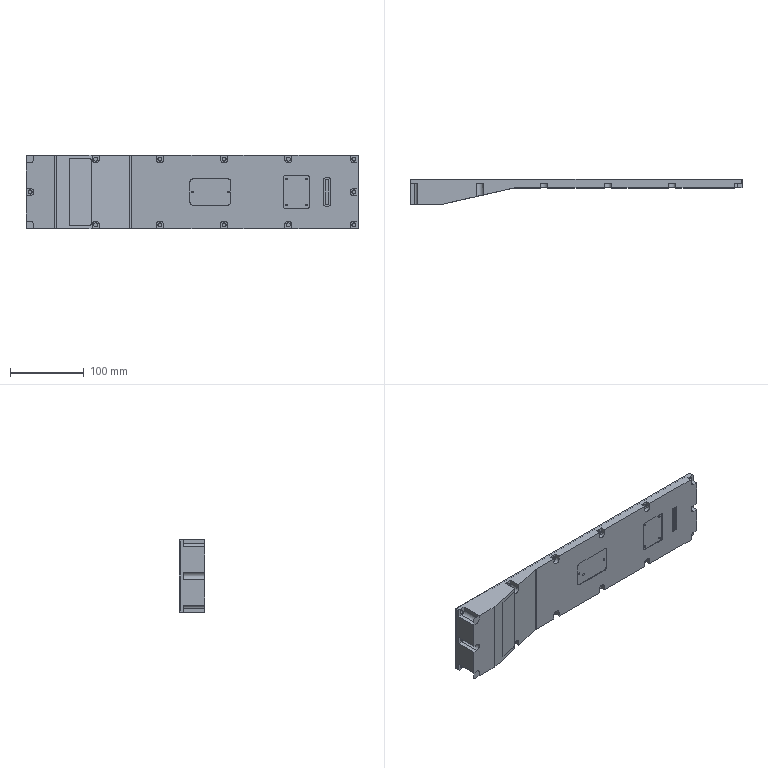NC program | Mastercam | posted with a generic post | part box 450 x 35 x 100 mm
Lines 35860 to 36211 of 140701:
(6 CHM |TOOL - 7|DIA. OFF. - 7|LEN. - 7|TOOL DIA. - 6.)
N2484 T7 M6
N2486 G0 G54 G90 X-179.894 Y-50.65 C0. B0. S7000 M3
N2488 G43 H7 Z50.
N2490 Z1.
N2492 G1 Z-.7 F600.
N2494 X-185.894 F1000.
N2496 X-214.5
N2498 X-224.
N2500 G2 X-224.46 Y-50.46 J.65
N2502 G1 X-225.46 Y-49.46
N2504 G2 X-225.65 Y-49. I.46 J.46
N2506 G1 Y49.
N2508 G2 X-225.46 Y49.46 I.65
N2510 G1 X-224.46 Y50.46
N2512 G2 X-224. Y50.65 I.46 J-.46
N2514 G1 X-214.5
N2516 X-185.894
N2518 X-179.894
N2520 G0 Z50.
N2522 X151.65 Y-50.6
N2524 Z1.
N2526 G1 Z-1.5 F600.
N2528 X152.25 F1000.
N2530 G3 X152.85 Y-50. J.6
N2532 G1 Y-40.
N2534 G2 X154. Y-38.85 I1.15
N2536 G1 X194.
N2538 G2 X195.15 Y-40. J-1.15
N2540 G1 Y-50.
N2542 G2 X194. Y-51.15 I-1.15
N2544 G1 X154.
N2546 G2 X152.85 Y-50. J1.15
N2548 G3 X152.25 Y-49.4 I-.6
N2550 G1 X151.65
N2552 G0 Z50.
N2554 X64.65 Y-50.6
N2556 Z1.
N2558 G1 Z-1.5 F600.
N2560 X65.25 F1000.
N2562 G3 X65.85 Y-50. J.6
N2564 G1 Y-40.
N2566 G2 X67. Y-38.85 I1.15
N2568 G1 X107.
N2570 G2 X108.15 Y-40. J-1.15
N2572 G1 Y-50.
N2574 G2 X107. Y-51.15 I-1.15
N2576 G1 X67.
N2578 G2 X65.85 Y-50. J1.15
N2580 G3 X65.25 Y-49.4 I-.6
N2582 G1 X64.65
N2584 G0 Z50.
N2586 X-22.35 Y-50.6
N2588 Z1.
N2590 G1 Z-1.5 F600.
N2592 X-21.75 F1000.
N2594 G3 X-21.15 Y-50. J.6
N2596 G1 Y-40.
N2598 G2 X-20. Y-38.85 I1.15
N2600 G1 X20.
N2602 G2 X21.15 Y-40. J-1.15
N2604 G1 Y-50.
N2606 G2 X20. Y-51.15 I-1.15
N2608 G1 X-20.
N2610 G2 X-21.15 Y-50. J1.15
N2612 G3 X-21.75 Y-49.4 I-.6
N2614 G1 X-22.35
N2616 G0 Z50.
N2618 X151.65 Y39.4
N2620 Z1.
N2622 G1 Z-1.5 F600.
N2624 X152.25 F1000.
N2626 G3 X152.85 Y40. J.6
N2628 G1 Y50.
N2630 G2 X154. Y51.15 I1.15
N2632 G1 X194.
N2634 G2 X195.15 Y50. J-1.15
N2636 G1 Y40.
N2638 G2 X194. Y38.85 I-1.15
N2640 G1 X154.
N2642 G2 X152.85 Y40. J1.15
N2644 G3 X152.25 Y40.6 I-.6
N2646 G1 X151.65
N2648 G0 Z50.
N2650 X64.65 Y39.4
N2652 Z1.
N2654 G1 Z-1.5 F600.
N2656 X65.25 F1000.
N2658 G3 X65.85 Y40. J.6
N2660 G1 Y50.
N2662 G2 X67. Y51.15 I1.15
N2664 G1 X107.
N2666 G2 X108.15 Y50. J-1.15
N2668 G1 Y40.
N2670 G2 X107. Y38.85 I-1.15
N2672 G1 X67.
N2674 G2 X65.85 Y40. J1.15
N2676 G3 X65.25 Y40.6 I-.6
N2678 G1 X64.65
N2680 G0 Z50.
N2682 X-22.35 Y39.4
N2684 Z1.
N2686 G1 Z-1.5 F600.
N2688 X-21.75 F1000.
N2690 G3 X-21.15 Y40. J.6
N2692 G1 Y50.
N2694 G2 X-20. Y51.15 I1.15
N2696 G1 X20.
N2698 G2 X21.15 Y50. J-1.15
N2700 G1 Y40.
N2702 G2 X20. Y38.85 I-1.15
N2704 G1 X-20.
N2706 G2 X-21.15 Y40. J1.15
N2708 G3 X-21.75 Y40.6 I-.6
N2710 G1 X-22.35
N2712 G0 Z50.
N2714 M5
N2716 G0 G28 G91 Z0.
N2718 G28
N2720 M01
N2722 G0 G17 G40 G80 G90 G94 G98
N2724 G0 G28 G91 Z0.
(100 FEM |TOOL - 24|DIA. OFF. - 24|LEN. - 24|TOOL DIA. - 100.)
M00
N2726 T24 M6
N2728 G0 G54 G90 X-339. Y22.498 C0. B0. S4000 M3
N2730 G43 H24 Z50.
N2732 Z2.
N2734 G1 Z0. F600.
N2736 X279. F1000.
N2738 G2 X301.498 Y0. J-22.498
N2740 X279. Y-22.498 I-22.498
N2742 G1 X-339.
N2744 G0 Z50.
N2746 M5
N2748 G0 G28 G91 Z0.
N2750 G28
N2752 M01
N2754 G0 G17 G40 G80 G90 G94 G98
N2756 G0 G28 G91 Z0.
(12 FEM |TOOL - 12|DIA. OFF. - 12|LEN. - 12|TOOL DIA. - 12.)
N2758 T12 M6
N2760 G0 G54 G90 X-220.6 Y-62.168 C0. B0. S7000 M3
N2762 G43 H12 Z50.
N2764 Z1.
N2766 G1 Z-12.55 F600.
N2768 X-229.085 Y-53.683 F1000.
N2770 X-229.384 Y-53.384
N2772 G2 X-231.2 Y-49. I4.384 J4.384
N2774 G1 Y49.
N2776 G2 X-229.384 Y53.384 I6.2
N2778 G1 X-228.384 Y54.384
N2780 G2 X-224. Y56.2 I4.384 J-4.384
N2782 G1 X224.
N2784 G2 X228.384 Y54.384 J-6.2
N2786 G1 X229.384 Y53.384
N2788 G2 X231.2 Y49. I-4.384 J-4.384
N2790 G1 Y-49.
N2792 G2 X229.384 Y-53.384 I-6.2
N2794 G1 X228.384 Y-54.384
N2796 G2 X224. Y-56.2 I-4.384 J4.384
N2798 G1 X-224.
N2800 G2 X-228.384 Y-54.384 J6.2
N2802 G1 X-229.085 Y-53.683
N2804 X-237.57 Y-45.198
N2806 G0 Z50.
N2808 X-220.6 Y-62.168
N2810 Z1.
N2812 G1 Z-12.55 F600.
N2814 X-229.085 Y-53.683 F1000.
N2816 X-229.384 Y-53.384
N2818 G2 X-231.2 Y-49. I4.384 J4.384
N2820 G1 Y49.
N2822 G2 X-229.384 Y53.384 I6.2
N2824 G1 X-228.384 Y54.384
N2826 G2 X-224. Y56.2 I4.384 J-4.384
N2828 G1 X224.
N2830 G2 X228.384 Y54.384 J-6.2
N2832 G1 X229.384 Y53.384
N2834 G2 X231.2 Y49. I-4.384 J-4.384
N2836 G1 Y-49.
N2838 G2 X229.384 Y-53.384 I-6.2
N2840 G1 X228.384 Y-54.384
N2842 G2 X224. Y-56.2 I-4.384 J4.384
N2844 G1 X-224.
N2846 G2 X-228.384 Y-54.384 J6.2
N2848 G1 X-229.085 Y-53.683
N2850 X-237.57 Y-45.198
N2852 G0 Z50.
N2854 X-220.6 Y-62.168
N2856 Z-11.55
N2858 G1 Z-25.1 F600.
N2860 X-229.085 Y-53.683 F1000.
N2862 X-229.384 Y-53.384
N2864 G2 X-231.2 Y-49. I4.384 J4.384
N2866 G1 Y49.
N2868 G2 X-229.384 Y53.384 I6.2
N2870 G1 X-228.384 Y54.384
N2872 G2 X-224. Y56.2 I4.384 J-4.384
N2874 G1 X224.
N2876 G2 X228.384 Y54.384 J-6.2
N2878 G1 X229.384 Y53.384
N2880 G2 X231.2 Y49. I-4.384 J-4.384
N2882 G1 Y-49.
N2884 G2 X229.384 Y-53.384 I-6.2
N2886 G1 X228.384 Y-54.384
N2888 G2 X224. Y-56.2 I-4.384 J4.384
N2890 G1 X-224.
N2892 G2 X-228.384 Y-54.384 J6.2
N2894 G1 X-229.085 Y-53.683
N2896 X-237.57 Y-45.198
N2898 G0 Z50.
N2900 X-220.6 Y-62.168
N2902 Z-11.55
N2904 G1 Z-25.1 F600.
N2906 X-229.085 Y-53.683 F1000.
N2908 X-229.384 Y-53.384
N2910 G2 X-231.2 Y-49. I4.384 J4.384
N2912 G1 Y49.
N2914 G2 X-229.384 Y53.384 I6.2
N2916 G1 X-228.384 Y54.384
N2918 G2 X-224. Y56.2 I4.384 J-4.384
N2920 G1 X224.
N2922 G2 X228.384 Y54.384 J-6.2
N2924 G1 X229.384 Y53.384
N2926 G2 X231.2 Y49. I-4.384 J-4.384
N2928 G1 Y-49.
N2930 G2 X229.384 Y-53.384 I-6.2
N2932 G1 X228.384 Y-54.384
N2934 G2 X224. Y-56.2 I-4.384 J4.384
N2936 G1 X-224.
N2938 G2 X-228.384 Y-54.384 J6.2
N2940 G1 X-229.085 Y-53.683
N2942 X-237.57 Y-45.198
N2944 G0 Z50.
N2946 X-220.6 Y-62.168
N2948 Z-24.1
N2950 G1 Z-37.65 F600.
N2952 X-229.085 Y-53.683 F1000.
N2954 X-229.384 Y-53.384
N2956 G2 X-231.2 Y-49. I4.384 J4.384
N2958 G1 Y49.
N2960 G2 X-229.384 Y53.384 I6.2
N2962 G1 X-228.384 Y54.384
N2964 G2 X-224. Y56.2 I4.384 J-4.384
N2966 G1 X224.
N2968 G2 X228.384 Y54.384 J-6.2
N2970 G1 X229.384 Y53.384
N2972 G2 X231.2 Y49. I-4.384 J-4.384
N2974 G1 Y-49.
N2976 G2 X229.384 Y-53.384 I-6.2
N2978 G1 X228.384 Y-54.384
N2980 G2 X224. Y-56.2 I-4.384 J4.384
N2982 G1 X-224.
N2984 G2 X-228.384 Y-54.384 J6.2
N2986 G1 X-229.085 Y-53.683
N2988 X-237.57 Y-45.198
N2990 G0 Z50.
N2992 X-220.6 Y-62.168
N2994 Z-24.1
N2996 G1 Z-37.65 F600.
N2998 X-229.085 Y-53.683 F1000.
N3000 X-229.384 Y-53.384
N3002 G2 X-231.2 Y-49. I4.384 J4.384
N3004 G1 Y49.
N3006 G2 X-229.384 Y53.384 I6.2
N3008 G1 X-228.384 Y54.384
N3010 G2 X-224. Y56.2 I4.384 J-4.384
N3012 G1 X224.
N3014 G2 X228.384 Y54.384 J-6.2
N3016 G1 X229.384 Y53.384
N3018 G2 X231.2 Y49. I-4.384 J-4.384
N3020 G1 Y-49.
N3022 G2 X229.384 Y-53.384 I-6.2
N3024 G1 X228.384 Y-54.384
N3026 G2 X224. Y-56.2 I-4.384 J4.384
N3028 G1 X-224.
N3030 G2 X-228.384 Y-54.384 J6.2
N3032 G1 X-229.085 Y-53.683
N3034 X-237.57 Y-45.198
N3036 G0 Z50.
N3038 M5
N3040 G0 G28 G91 Z0.
N3042 G28
N3044 M01
N3046 G0 G17 G40 G80 G90 G94 G98
N3048 G0 G28 G91 Z0.
(100 FEM |TOOL - 24|DIA. OFF. - 24|LEN. - 24|TOOL DIA. - 100.)
N3050 T24 M6
N3052 G0 G54 G90 X-339. Y22.498 C0. B0. S4000 M3
N3054 G43 H24 Z53.
N3056 Z5.
N3058 G1 Z2.533 F600.
N3060 X279. F3000.
N3062 G2 X301.498 Y0. J-22.498
N3064 X279. Y-22.498 I-22.498
N3066 G1 X-339.
N3068 G0 Z52.533
N3070 Y22.498
N3072 Z4.533
N3074 G1 Z2.067 F600.
N3076 X279. F3000.
N3078 G2 X301.498 Y0. J-22.498
N3080 X279. Y-22.498 I-22.498
N3082 G1 X-339.
N3084 G0 Z52.067
N3086 Y22.498
N3088 Z4.067
N3090 G1 Z1.6 F600.
N3092 X279. F3000.
N3094 G2 X301.498 Y0. J-22.498
N3096 X279. Y-22.498 I-22.498
N3098 G1 X-339.
N3100 G0 Z51.6
N3102 Y22.498
N3104 Z3.6
N3106 G1 Z1.133 F600.
N3108 X279. F3000.
N3110 G2 X301.498 Y0. J-22.498
N3112 X279. Y-22.498 I-22.498
N3114 G1 X-339.
N3116 G0 Z51.133
N3118 Y22.498
N3120 Z3.133
N3122 G1 Z.667 F600.
N3124 X279. F3000.
N3126 G2 X301.498 Y0. J-22.498
N3128 X279. Y-22.498 I-22.498
N3130 G1 X-339.
N3132 G0 Z50.667
N3134 Y22.498
N3136 Z2.667
N3138 G1 Z.2 F600.
N3140 X279. F3000.
N3142 G2 X301.498 Y0. J-22.498
N3144 X279. Y-22.498 I-22.498
N3146 G1 X-339.
N3148 G0 Z50.2
N3150 Y22.498
N3152 Z2.2
N3154 G1 Z.1 F600.
N3156 X279. F1000.
N3158 G2 X301.498 Y0. J-22.498
N3160 X279. Y-22.498 I-22.498
N3162 G1 X-339.
N3164 G0 Z50.1
N3166 M5
N3168 G0 G28 G91 Z0.
N3170 G28
N3172 M01
N3174 G0 G17 G40 G80 G90 G94 G98
N3176 G0 G28 G91 Z0.